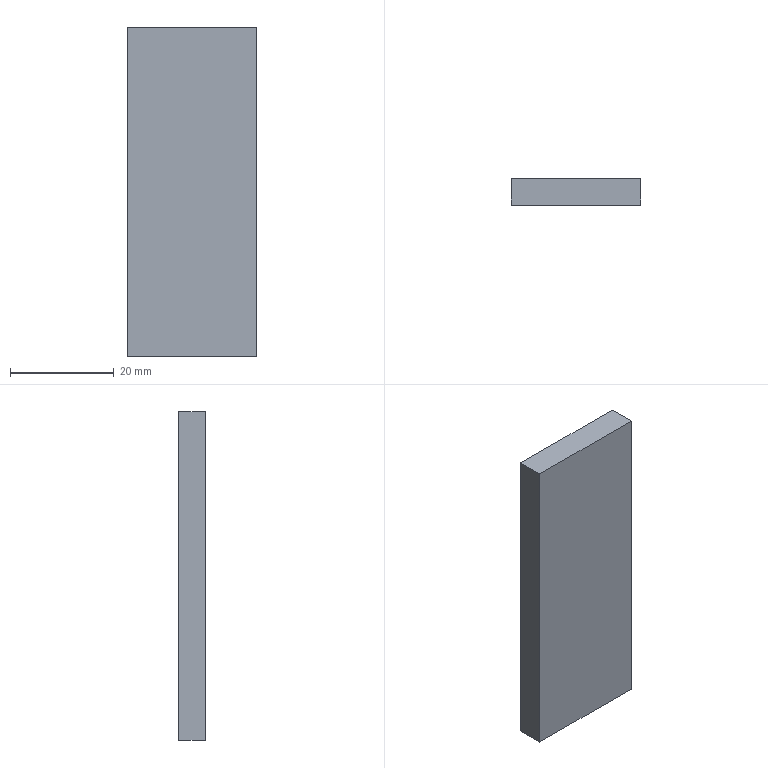Part | STEP file | 0245_Z_103_UM25-8YU-232-SCNUW_1 | 1 solid | 6 faces | box 25 x 5.2 x 63.25 mm | volume 8222 mm3 | plane 6
STEP:
#1=CARTESIAN_POINT('',(0.,0.,0.));
#2=DIRECTION('',(0.,0.,1.));
#3=DIRECTION('',(1.,0.,0.));
#4=AXIS2_PLACEMENT_3D('',#1,#2,#3);
#5=CARTESIAN_POINT('',(-12.5,5.2,0.));
#6=VERTEX_POINT('',#5);
#7=CARTESIAN_POINT('',(-12.5,0.,0.));
#8=VERTEX_POINT('',#7);
#9=CARTESIAN_POINT('',(-12.5,0.,0.));
#10=DIRECTION('',(0.,-1.,0.));
#11=VECTOR('',#10,1.);
#12=LINE('',#9,#11);
#13=CARTESIAN_POINT('',(12.5,0.,0.));
#14=DIRECTION('',(0.,0.,-1.));
#15=DIRECTION('',(-1.,0.,0.));
#16=AXIS2_PLACEMENT_3D('',#13,#14,#15);
#17=PLANE('',#16);
#18=CARTESIAN_POINT('',(25.,0.));
#19=DIRECTION('',(0.,-1.));
#20=VECTOR('',#19,1.);
#21=LINE('',#18,#20);
#22=(GEOMETRIC_REPRESENTATION_CONTEXT(2)PARAMETRIC_REPRESENTATION_CONTEXT()REPRESENTATION_CONTEXT('',''));
#23=DEFINITIONAL_REPRESENTATION('',(#21),#22);
#24=PCURVE('',#17,#23);
#25=CARTESIAN_POINT('',(-12.5,5.2,0.));
#26=DIRECTION('',(-1.,0.,0.));
#27=DIRECTION('',(0.,0.,1.));
#28=AXIS2_PLACEMENT_3D('',#25,#26,#27);
#29=PLANE('',#28);
#30=CARTESIAN_POINT('',(0.,-5.2));
#31=DIRECTION('',(0.,-1.));
#32=VECTOR('',#31,1.);
#33=LINE('',#30,#32);
#34=(GEOMETRIC_REPRESENTATION_CONTEXT(2)PARAMETRIC_REPRESENTATION_CONTEXT()REPRESENTATION_CONTEXT('',''));
#35=DEFINITIONAL_REPRESENTATION('',(#33),#34);
#36=PCURVE('',#29,#35);
#37=SURFACE_CURVE('',#12,(#24,#36),.PCURVE_S1.);
#38=EDGE_CURVE('',#6,#8,#37,.T.);
#39=ORIENTED_EDGE('',*,*,#38,.T.);
#40=CARTESIAN_POINT('',(12.5,0.,0.));
#41=VERTEX_POINT('',#40);
#42=CARTESIAN_POINT('',(12.5,0.,0.));
#43=DIRECTION('',(-1.,0.,0.));
#44=VECTOR('',#43,1.);
#45=LINE('',#42,#44);
#46=CARTESIAN_POINT('',(0.,0.));
#47=DIRECTION('',(1.,0.));
#48=VECTOR('',#47,1.);
#49=LINE('',#46,#48);
#50=(GEOMETRIC_REPRESENTATION_CONTEXT(2)PARAMETRIC_REPRESENTATION_CONTEXT()REPRESENTATION_CONTEXT('',''));
#51=DEFINITIONAL_REPRESENTATION('',(#49),#50);
#52=PCURVE('',#17,#51);
#53=CARTESIAN_POINT('',(12.5,0.,0.));
#54=DIRECTION('',(0.,1.,0.));
#55=DIRECTION('',(0.,0.,1.));
#56=AXIS2_PLACEMENT_3D('',#53,#54,#55);
#57=PLANE('',#56);
#58=CARTESIAN_POINT('',(0.,0.));
#59=DIRECTION('',(0.,-1.));
#60=VECTOR('',#59,1.);
#61=LINE('',#58,#60);
#62=(GEOMETRIC_REPRESENTATION_CONTEXT(2)PARAMETRIC_REPRESENTATION_CONTEXT()REPRESENTATION_CONTEXT('',''));
#63=DEFINITIONAL_REPRESENTATION('',(#61),#62);
#64=PCURVE('',#57,#63);
#65=SURFACE_CURVE('',#45,(#52,#64),.PCURVE_S1.);
#66=EDGE_CURVE('',#41,#8,#65,.T.);
#67=ORIENTED_EDGE('',*,*,#66,.F.);
#68=CARTESIAN_POINT('',(12.5,5.2,0.));
#69=VERTEX_POINT('',#68);
#70=CARTESIAN_POINT('',(12.5,0.,0.));
#71=DIRECTION('',(0.,-1.,0.));
#72=VECTOR('',#71,1.);
#73=LINE('',#70,#72);
#74=CARTESIAN_POINT('',(0.,0.));
#75=DIRECTION('',(0.,-1.));
#76=VECTOR('',#75,1.);
#77=LINE('',#74,#76);
#78=(GEOMETRIC_REPRESENTATION_CONTEXT(2)PARAMETRIC_REPRESENTATION_CONTEXT()REPRESENTATION_CONTEXT('',''));
#79=DEFINITIONAL_REPRESENTATION('',(#77),#78);
#80=PCURVE('',#17,#79);
#81=CARTESIAN_POINT('',(12.5,5.2,0.));
#82=DIRECTION('',(-1.,0.,0.));
#83=DIRECTION('',(0.,0.,1.));
#84=AXIS2_PLACEMENT_3D('',#81,#82,#83);
#85=PLANE('',#84);
#86=CARTESIAN_POINT('',(0.,-5.2));
#87=DIRECTION('',(0.,-1.));
#88=VECTOR('',#87,1.);
#89=LINE('',#86,#88);
#90=(GEOMETRIC_REPRESENTATION_CONTEXT(2)PARAMETRIC_REPRESENTATION_CONTEXT()REPRESENTATION_CONTEXT('',''));
#91=DEFINITIONAL_REPRESENTATION('',(#89),#90);
#92=PCURVE('',#85,#91);
#93=SURFACE_CURVE('',#73,(#80,#92),.PCURVE_S1.);
#94=EDGE_CURVE('',#69,#41,#93,.T.);
#95=ORIENTED_EDGE('',*,*,#94,.F.);
#96=CARTESIAN_POINT('',(12.5,5.2,0.));
#97=DIRECTION('',(-1.,0.,0.));
#98=VECTOR('',#97,1.);
#99=LINE('',#96,#98);
#100=CARTESIAN_POINT('',(0.,5.2));
#101=DIRECTION('',(1.,0.));
#102=VECTOR('',#101,1.);
#103=LINE('',#100,#102);
#104=(GEOMETRIC_REPRESENTATION_CONTEXT(2)PARAMETRIC_REPRESENTATION_CONTEXT()REPRESENTATION_CONTEXT('',''));
#105=DEFINITIONAL_REPRESENTATION('',(#103),#104);
#106=PCURVE('',#17,#105);
#107=CARTESIAN_POINT('',(12.5,5.2,0.));
#108=DIRECTION('',(0.,-1.,0.));
#109=DIRECTION('',(0.,0.,-1.));
#110=AXIS2_PLACEMENT_3D('',#107,#108,#109);
#111=PLANE('',#110);
#112=CARTESIAN_POINT('',(0.,0.));
#113=DIRECTION('',(0.,-1.));
#114=VECTOR('',#113,1.);
#115=LINE('',#112,#114);
#116=(GEOMETRIC_REPRESENTATION_CONTEXT(2)PARAMETRIC_REPRESENTATION_CONTEXT()REPRESENTATION_CONTEXT('',''));
#117=DEFINITIONAL_REPRESENTATION('',(#115),#116);
#118=PCURVE('',#111,#117);
#119=SURFACE_CURVE('',#99,(#106,#118),.PCURVE_S1.);
#120=EDGE_CURVE('',#69,#6,#119,.T.);
#121=ORIENTED_EDGE('',*,*,#120,.T.);
#122=EDGE_LOOP('',(#39,#67,#95,#121));
#123=FACE_BOUND('',#122,.T.);
#124=ADVANCED_FACE('',(#123),#17,.F.);
#125=CARTESIAN_POINT('',(-12.5,0.,-63.25));
#126=VERTEX_POINT('',#125);
#127=CARTESIAN_POINT('',(-12.5,0.,0.));
#128=DIRECTION('',(0.,0.,-1.));
#129=VECTOR('',#128,1.);
#130=LINE('',#127,#129);
#131=CARTESIAN_POINT('',(0.,-25.));
#132=DIRECTION('',(-1.,0.));
#133=VECTOR('',#132,1.);
#134=LINE('',#131,#133);
#135=(GEOMETRIC_REPRESENTATION_CONTEXT(2)PARAMETRIC_REPRESENTATION_CONTEXT()REPRESENTATION_CONTEXT('',''));
#136=DEFINITIONAL_REPRESENTATION('',(#134),#135);
#137=PCURVE('',#57,#136);
#138=CARTESIAN_POINT('',(0.,-5.2));
#139=DIRECTION('',(-1.,0.));
#140=VECTOR('',#139,1.);
#141=LINE('',#138,#140);
#142=(GEOMETRIC_REPRESENTATION_CONTEXT(2)PARAMETRIC_REPRESENTATION_CONTEXT()REPRESENTATION_CONTEXT('',''));
#143=DEFINITIONAL_REPRESENTATION('',(#141),#142);
#144=PCURVE('',#29,#143);
#145=SURFACE_CURVE('',#130,(#137,#144),.PCURVE_S1.);
#146=EDGE_CURVE('',#8,#126,#145,.T.);
#147=ORIENTED_EDGE('',*,*,#146,.T.);
#148=CARTESIAN_POINT('',(12.5,0.,-63.25));
#149=VERTEX_POINT('',#148);
#150=CARTESIAN_POINT('',(12.5,0.,-63.25));
#151=DIRECTION('',(-1.,0.,0.));
#152=VECTOR('',#151,1.);
#153=LINE('',#150,#152);
#154=CARTESIAN_POINT('',(-63.25,0.));
#155=DIRECTION('',(0.,-1.));
#156=VECTOR('',#155,1.);
#157=LINE('',#154,#156);
#158=(GEOMETRIC_REPRESENTATION_CONTEXT(2)PARAMETRIC_REPRESENTATION_CONTEXT()REPRESENTATION_CONTEXT('',''));
#159=DEFINITIONAL_REPRESENTATION('',(#157),#158);
#160=PCURVE('',#57,#159);
#161=CARTESIAN_POINT('',(12.5,0.,-63.25));
#162=DIRECTION('',(0.,0.,1.));
#163=DIRECTION('',(1.,0.,0.));
#164=AXIS2_PLACEMENT_3D('',#161,#162,#163);
#165=PLANE('',#164);
#166=CARTESIAN_POINT('',(0.,0.));
#167=DIRECTION('',(-1.,0.));
#168=VECTOR('',#167,1.);
#169=LINE('',#166,#168);
#170=(GEOMETRIC_REPRESENTATION_CONTEXT(2)PARAMETRIC_REPRESENTATION_CONTEXT()REPRESENTATION_CONTEXT('',''));
#171=DEFINITIONAL_REPRESENTATION('',(#169),#170);
#172=PCURVE('',#165,#171);
#173=SURFACE_CURVE('',#153,(#160,#172),.PCURVE_S1.);
#174=EDGE_CURVE('',#149,#126,#173,.T.);
#175=ORIENTED_EDGE('',*,*,#174,.F.);
#176=CARTESIAN_POINT('',(12.5,0.,0.));
#177=DIRECTION('',(0.,0.,-1.));
#178=VECTOR('',#177,1.);
#179=LINE('',#176,#178);
#180=CARTESIAN_POINT('',(0.,0.));
#181=DIRECTION('',(-1.,0.));
#182=VECTOR('',#181,1.);
#183=LINE('',#180,#182);
#184=(GEOMETRIC_REPRESENTATION_CONTEXT(2)PARAMETRIC_REPRESENTATION_CONTEXT()REPRESENTATION_CONTEXT('',''));
#185=DEFINITIONAL_REPRESENTATION('',(#183),#184);
#186=PCURVE('',#57,#185);
#187=CARTESIAN_POINT('',(0.,-5.2));
#188=DIRECTION('',(-1.,0.));
#189=VECTOR('',#188,1.);
#190=LINE('',#187,#189);
#191=(GEOMETRIC_REPRESENTATION_CONTEXT(2)PARAMETRIC_REPRESENTATION_CONTEXT()REPRESENTATION_CONTEXT('',''));
#192=DEFINITIONAL_REPRESENTATION('',(#190),#191);
#193=PCURVE('',#85,#192);
#194=SURFACE_CURVE('',#179,(#186,#193),.PCURVE_S1.);
#195=EDGE_CURVE('',#41,#149,#194,.T.);
#196=ORIENTED_EDGE('',*,*,#195,.F.);
#197=ORIENTED_EDGE('',*,*,#66,.T.);
#198=EDGE_LOOP('',(#147,#175,#196,#197));
#199=FACE_BOUND('',#198,.T.);
#200=ADVANCED_FACE('',(#199),#57,.F.);
#201=CARTESIAN_POINT('',(-12.5,5.2,-63.25));
#202=VERTEX_POINT('',#201);
#203=CARTESIAN_POINT('',(-12.5,0.,-63.25));
#204=DIRECTION('',(0.,1.,0.));
#205=VECTOR('',#204,1.);
#206=LINE('',#203,#205);
#207=CARTESIAN_POINT('',(-25.,0.));
#208=DIRECTION('',(0.,1.));
#209=VECTOR('',#208,1.);
#210=LINE('',#207,#209);
#211=(GEOMETRIC_REPRESENTATION_CONTEXT(2)PARAMETRIC_REPRESENTATION_CONTEXT()REPRESENTATION_CONTEXT('',''));
#212=DEFINITIONAL_REPRESENTATION('',(#210),#211);
#213=PCURVE('',#165,#212);
#214=CARTESIAN_POINT('',(-63.25,-5.2));
#215=DIRECTION('',(0.,1.));
#216=VECTOR('',#215,1.);
#217=LINE('',#214,#216);
#218=(GEOMETRIC_REPRESENTATION_CONTEXT(2)PARAMETRIC_REPRESENTATION_CONTEXT()REPRESENTATION_CONTEXT('',''));
#219=DEFINITIONAL_REPRESENTATION('',(#217),#218);
#220=PCURVE('',#29,#219);
#221=SURFACE_CURVE('',#206,(#213,#220),.PCURVE_S1.);
#222=EDGE_CURVE('',#126,#202,#221,.T.);
#223=ORIENTED_EDGE('',*,*,#222,.T.);
#224=CARTESIAN_POINT('',(12.5,5.2,-63.25));
#225=VERTEX_POINT('',#224);
#226=CARTESIAN_POINT('',(12.5,5.2,-63.25));
#227=DIRECTION('',(-1.,0.,0.));
#228=VECTOR('',#227,1.);
#229=LINE('',#226,#228);
#230=CARTESIAN_POINT('',(0.,5.2));
#231=DIRECTION('',(-1.,0.));
#232=VECTOR('',#231,1.);
#233=LINE('',#230,#232);
#234=(GEOMETRIC_REPRESENTATION_CONTEXT(2)PARAMETRIC_REPRESENTATION_CONTEXT()REPRESENTATION_CONTEXT('',''));
#235=DEFINITIONAL_REPRESENTATION('',(#233),#234);
#236=PCURVE('',#165,#235);
#237=CARTESIAN_POINT('',(63.25,0.));
#238=DIRECTION('',(0.,-1.));
#239=VECTOR('',#238,1.);
#240=LINE('',#237,#239);
#241=(GEOMETRIC_REPRESENTATION_CONTEXT(2)PARAMETRIC_REPRESENTATION_CONTEXT()REPRESENTATION_CONTEXT('',''));
#242=DEFINITIONAL_REPRESENTATION('',(#240),#241);
#243=PCURVE('',#111,#242);
#244=SURFACE_CURVE('',#229,(#236,#243),.PCURVE_S1.);
#245=EDGE_CURVE('',#225,#202,#244,.T.);
#246=ORIENTED_EDGE('',*,*,#245,.F.);
#247=CARTESIAN_POINT('',(12.5,0.,-63.25));
#248=DIRECTION('',(0.,1.,0.));
#249=VECTOR('',#248,1.);
#250=LINE('',#247,#249);
#251=CARTESIAN_POINT('',(0.,0.));
#252=DIRECTION('',(0.,1.));
#253=VECTOR('',#252,1.);
#254=LINE('',#251,#253);
#255=(GEOMETRIC_REPRESENTATION_CONTEXT(2)PARAMETRIC_REPRESENTATION_CONTEXT()REPRESENTATION_CONTEXT('',''));
#256=DEFINITIONAL_REPRESENTATION('',(#254),#255);
#257=PCURVE('',#165,#256);
#258=CARTESIAN_POINT('',(-63.25,-5.2));
#259=DIRECTION('',(0.,1.));
#260=VECTOR('',#259,1.);
#261=LINE('',#258,#260);
#262=(GEOMETRIC_REPRESENTATION_CONTEXT(2)PARAMETRIC_REPRESENTATION_CONTEXT()REPRESENTATION_CONTEXT('',''));
#263=DEFINITIONAL_REPRESENTATION('',(#261),#262);
#264=PCURVE('',#85,#263);
#265=SURFACE_CURVE('',#250,(#257,#264),.PCURVE_S1.);
#266=EDGE_CURVE('',#149,#225,#265,.T.);
#267=ORIENTED_EDGE('',*,*,#266,.F.);
#268=ORIENTED_EDGE('',*,*,#174,.T.);
#269=EDGE_LOOP('',(#223,#246,#267,#268));
#270=FACE_BOUND('',#269,.T.);
#271=ADVANCED_FACE('',(#270),#165,.F.);
#272=CARTESIAN_POINT('',(-12.5,5.2,0.));
#273=DIRECTION('',(0.,0.,1.));
#274=VECTOR('',#273,1.);
#275=LINE('',#272,#274);
#276=CARTESIAN_POINT('',(0.,-25.));
#277=DIRECTION('',(-1.,0.));
#278=VECTOR('',#277,1.);
#279=LINE('',#276,#278);
#280=(GEOMETRIC_REPRESENTATION_CONTEXT(2)PARAMETRIC_REPRESENTATION_CONTEXT()REPRESENTATION_CONTEXT('',''));
#281=DEFINITIONAL_REPRESENTATION('',(#279),#280);
#282=PCURVE('',#111,#281);
#283=CARTESIAN_POINT('',(0.,0.));
#284=DIRECTION('',(1.,0.));
#285=VECTOR('',#284,1.);
#286=LINE('',#283,#285);
#287=(GEOMETRIC_REPRESENTATION_CONTEXT(2)PARAMETRIC_REPRESENTATION_CONTEXT()REPRESENTATION_CONTEXT('',''));
#288=DEFINITIONAL_REPRESENTATION('',(#286),#287);
#289=PCURVE('',#29,#288);
#290=SURFACE_CURVE('',#275,(#282,#289),.PCURVE_S1.);
#291=EDGE_CURVE('',#202,#6,#290,.T.);
#292=ORIENTED_EDGE('',*,*,#291,.T.);
#293=ORIENTED_EDGE('',*,*,#120,.F.);
#294=CARTESIAN_POINT('',(12.5,5.2,0.));
#295=DIRECTION('',(0.,0.,1.));
#296=VECTOR('',#295,1.);
#297=LINE('',#294,#296);
#298=CARTESIAN_POINT('',(0.,0.));
#299=DIRECTION('',(-1.,0.));
#300=VECTOR('',#299,1.);
#301=LINE('',#298,#300);
#302=(GEOMETRIC_REPRESENTATION_CONTEXT(2)PARAMETRIC_REPRESENTATION_CONTEXT()REPRESENTATION_CONTEXT('',''));
#303=DEFINITIONAL_REPRESENTATION('',(#301),#302);
#304=PCURVE('',#111,#303);
#305=CARTESIAN_POINT('',(0.,0.));
#306=DIRECTION('',(1.,0.));
#307=VECTOR('',#306,1.);
#308=LINE('',#305,#307);
#309=(GEOMETRIC_REPRESENTATION_CONTEXT(2)PARAMETRIC_REPRESENTATION_CONTEXT()REPRESENTATION_CONTEXT('',''));
#310=DEFINITIONAL_REPRESENTATION('',(#308),#309);
#311=PCURVE('',#85,#310);
#312=SURFACE_CURVE('',#297,(#304,#311),.PCURVE_S1.);
#313=EDGE_CURVE('',#225,#69,#312,.T.);
#314=ORIENTED_EDGE('',*,*,#313,.F.);
#315=ORIENTED_EDGE('',*,*,#245,.T.);
#316=EDGE_LOOP('',(#292,#293,#314,#315));
#317=FACE_BOUND('',#316,.T.);
#318=ADVANCED_FACE('',(#317),#111,.F.);
#319=ORIENTED_EDGE('',*,*,#94,.T.);
#320=ORIENTED_EDGE('',*,*,#195,.T.);
#321=ORIENTED_EDGE('',*,*,#266,.T.);
#322=ORIENTED_EDGE('',*,*,#313,.T.);
#323=EDGE_LOOP('',(#319,#320,#321,#322));
#324=FACE_BOUND('',#323,.T.);
#325=ADVANCED_FACE('',(#324),#85,.F.);
#326=ORIENTED_EDGE('',*,*,#38,.F.);
#327=ORIENTED_EDGE('',*,*,#291,.F.);
#328=ORIENTED_EDGE('',*,*,#222,.F.);
#329=ORIENTED_EDGE('',*,*,#146,.F.);
#330=EDGE_LOOP('',(#326,#327,#328,#329));
#331=FACE_BOUND('',#330,.T.);
#332=ADVANCED_FACE('',(#331),#29,.T.);
#333=CLOSED_SHELL('',(#124,#200,#271,#318,#325,#332));
#334=MANIFOLD_SOLID_BREP('',#333);
#335=(LENGTH_UNIT()NAMED_UNIT(*)SI_UNIT(.MILLI.,.METRE.));
#336=UNCERTAINTY_MEASURE_WITH_UNIT(LENGTH_MEASURE(0.0000001),#335,'','');
#337=(NAMED_UNIT(*)PLANE_ANGLE_UNIT()SI_UNIT($,.RADIAN.));
#338=(NAMED_UNIT(*)SI_UNIT($,.STERADIAN.)SOLID_ANGLE_UNIT());
#339=(GEOMETRIC_REPRESENTATION_CONTEXT(3)GLOBAL_UNCERTAINTY_ASSIGNED_CONTEXT((#336))GLOBAL_UNIT_ASSIGNED_CONTEXT((#335,#337,#338))REPRESENTATION_CONTEXT('',''));
#340=ADVANCED_BREP_SHAPE_REPRESENTATION('',(#4,#334),#339);